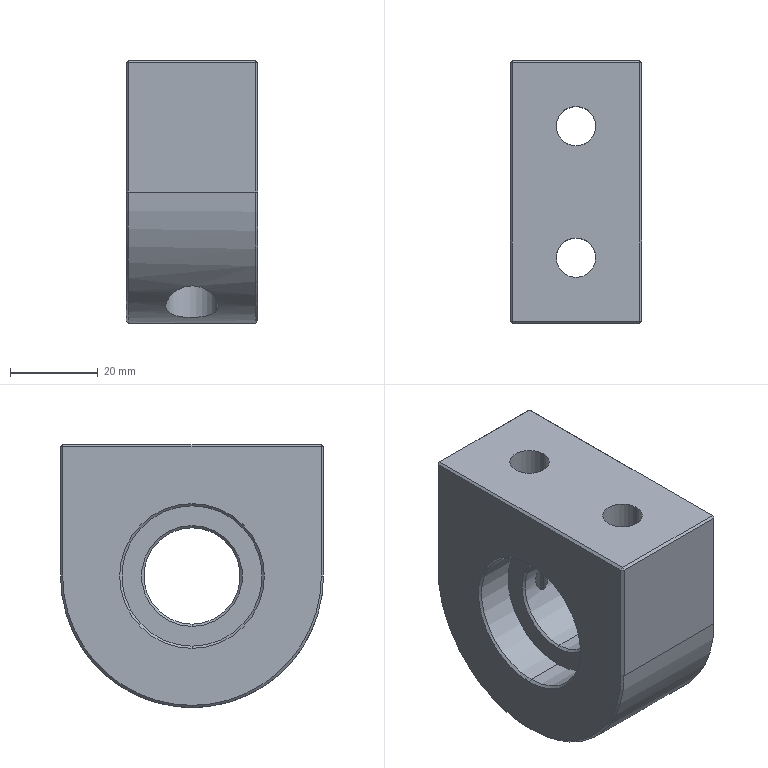Part | STEP file | PN_0009 hoist driving shaft fixing plate_Default | 1 solid | 42 faces | box 30 x 60 x 60 mm | volume 72459 mm3 | plane 20 | cylinder 13 | cone 9 | commonest cylinder face diameters 9 x4 12 x4 22 x2 32 x2 60 x1